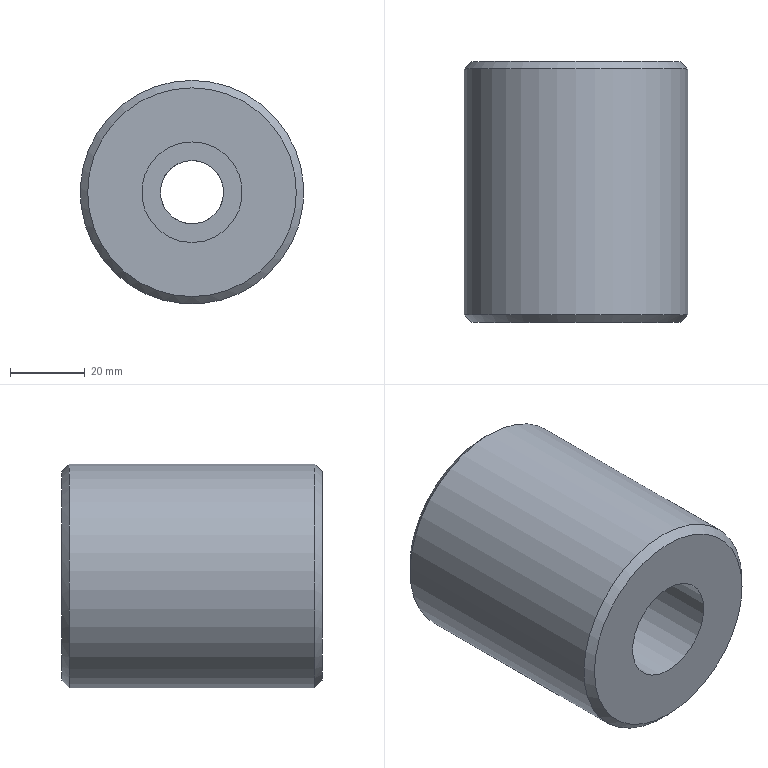Part | STEP file | 车灯-后视镜_id450_x_t | 1 solid | 8 faces | box 60 x 70 x 60 mm | volume 173692 mm3 | plane 3 | cylinder 3 | cone 2 | commonest cylinder face diameters 17 x1 27 x1 60 x1
STEP:
#1=CARTESIAN_POINT('',(165.,-345.,131.5));
#2=VERTEX_POINT('',#1);
#3=CARTESIAN_POINT('',(165.,-345.,159.5));
#4=DIRECTION('',(0.,1.,0.));
#5=DIRECTION('',(0.,0.,-1.));
#6=AXIS2_PLACEMENT_3D('',#3,#4,#5);
#7=CIRCLE('',#6,28.);
#8=EDGE_CURVE('',#2,#2,#7,.T.);
#9=ORIENTED_EDGE('',*,*,#8,.F.);
#10=EDGE_LOOP('',(#9));
#11=FACE_BOUND('',#10,.T.);
#12=CARTESIAN_POINT('',(165.,-345.,146.));
#13=VERTEX_POINT('',#12);
#14=CARTESIAN_POINT('',(165.,-345.,159.5));
#15=DIRECTION('',(0.,1.,0.));
#16=DIRECTION('',(0.,0.,-1.));
#17=AXIS2_PLACEMENT_3D('',#14,#15,#16);
#18=CIRCLE('',#17,13.5);
#19=EDGE_CURVE('',#13,#13,#18,.T.);
#20=ORIENTED_EDGE('',*,*,#19,.T.);
#21=EDGE_LOOP('',(#20));
#22=FACE_BOUND('',#21,.T.);
#23=CARTESIAN_POINT('',(165.,-345.,159.5));
#24=DIRECTION('',(0.,-1.,0.));
#25=DIRECTION('',(0.,0.,-1.));
#26=AXIS2_PLACEMENT_3D('',#23,#24,#25);
#27=PLANE('',#26);
#28=ADVANCED_FACE('',(#11,#22),#27,.T.);
#29=CARTESIAN_POINT('',(165.,-275.,187.5));
#30=VERTEX_POINT('',#29);
#31=CARTESIAN_POINT('',(165.,-275.,159.5));
#32=DIRECTION('',(0.,-1.,0.));
#33=DIRECTION('',(0.,0.,1.));
#34=AXIS2_PLACEMENT_3D('',#31,#32,#33);
#35=CIRCLE('',#34,28.);
#36=EDGE_CURVE('',#30,#30,#35,.T.);
#37=ORIENTED_EDGE('',*,*,#36,.F.);
#38=EDGE_LOOP('',(#37));
#39=FACE_BOUND('',#38,.T.);
#40=CARTESIAN_POINT('',(173.5,-275.,159.5));
#41=VERTEX_POINT('',#40);
#42=CARTESIAN_POINT('',(165.,-275.,159.5));
#43=DIRECTION('',(0.,1.,0.));
#44=DIRECTION('',(1.,0.,0.));
#45=AXIS2_PLACEMENT_3D('',#42,#43,#44);
#46=CIRCLE('',#45,8.5);
#47=EDGE_CURVE('',#41,#41,#46,.T.);
#48=ORIENTED_EDGE('',*,*,#47,.F.);
#49=EDGE_LOOP('',(#48));
#50=FACE_BOUND('',#49,.T.);
#51=CARTESIAN_POINT('',(165.,-275.,159.5));
#52=DIRECTION('',(0.,1.,0.));
#53=DIRECTION('',(0.,0.,1.));
#54=AXIS2_PLACEMENT_3D('',#51,#52,#53);
#55=PLANE('',#54);
#56=ADVANCED_FACE('',(#39,#50),#55,.T.);
#57=CARTESIAN_POINT('',(165.,-277.,189.5));
#58=VERTEX_POINT('',#57);
#59=CARTESIAN_POINT('',(165.,-277.,159.5));
#60=DIRECTION('',(0.,1.,0.));
#61=DIRECTION('',(0.,0.,1.));
#62=AXIS2_PLACEMENT_3D('',#59,#60,#61);
#63=CIRCLE('',#62,30.);
#64=EDGE_CURVE('',#58,#58,#63,.T.);
#65=ORIENTED_EDGE('',*,*,#64,.F.);
#66=EDGE_LOOP('',(#65));
#67=FACE_BOUND('',#66,.T.);
#68=CARTESIAN_POINT('',(165.,-343.,189.5));
#69=VERTEX_POINT('',#68);
#70=CARTESIAN_POINT('',(165.,-343.,159.5));
#71=DIRECTION('',(0.,-1.,0.));
#72=DIRECTION('',(0.,0.,1.));
#73=AXIS2_PLACEMENT_3D('',#70,#71,#72);
#74=CIRCLE('',#73,30.);
#75=EDGE_CURVE('',#69,#69,#74,.T.);
#76=ORIENTED_EDGE('',*,*,#75,.F.);
#77=EDGE_LOOP('',(#76));
#78=FACE_BOUND('',#77,.T.);
#79=CARTESIAN_POINT('',(165.,-275.,159.5));
#80=DIRECTION('',(0.,-1.,0.));
#81=DIRECTION('',(0.,0.,-1.));
#82=AXIS2_PLACEMENT_3D('',#79,#80,#81);
#83=CYLINDRICAL_SURFACE('',#82,30.);
#84=ADVANCED_FACE('',(#67,#78),#83,.T.);
#85=CARTESIAN_POINT('',(165.,-323.,168.));
#86=VERTEX_POINT('',#85);
#87=CARTESIAN_POINT('',(165.,-323.,159.5));
#88=DIRECTION('',(0.,1.,0.));
#89=DIRECTION('',(0.,0.,1.));
#90=AXIS2_PLACEMENT_3D('',#87,#88,#89);
#91=CIRCLE('',#90,8.5);
#92=EDGE_CURVE('',#86,#86,#91,.T.);
#93=ORIENTED_EDGE('',*,*,#92,.F.);
#94=EDGE_LOOP('',(#93));
#95=FACE_BOUND('',#94,.T.);
#96=ORIENTED_EDGE('',*,*,#47,.T.);
#97=EDGE_LOOP('',(#96));
#98=FACE_BOUND('',#97,.T.);
#99=CARTESIAN_POINT('',(165.,-275.,159.5));
#100=DIRECTION('',(0.,-1.,0.));
#101=DIRECTION('',(1.,0.,0.));
#102=AXIS2_PLACEMENT_3D('',#99,#100,#101);
#103=CYLINDRICAL_SURFACE('',#102,8.5);
#104=ADVANCED_FACE('',(#95,#98),#103,.F.);
#105=ORIENTED_EDGE('',*,*,#92,.T.);
#106=EDGE_LOOP('',(#105));
#107=FACE_BOUND('',#106,.T.);
#108=CARTESIAN_POINT('',(165.,-323.,173.));
#109=VERTEX_POINT('',#108);
#110=CARTESIAN_POINT('',(165.,-323.,159.5));
#111=DIRECTION('',(0.,1.,0.));
#112=DIRECTION('',(0.,0.,1.));
#113=AXIS2_PLACEMENT_3D('',#110,#111,#112);
#114=CIRCLE('',#113,13.5);
#115=EDGE_CURVE('',#109,#109,#114,.T.);
#116=ORIENTED_EDGE('',*,*,#115,.F.);
#117=EDGE_LOOP('',(#116));
#118=FACE_BOUND('',#117,.T.);
#119=CARTESIAN_POINT('',(165.,-323.,159.5));
#120=DIRECTION('',(0.,1.,0.));
#121=DIRECTION('',(-1.,0.,0.));
#122=AXIS2_PLACEMENT_3D('',#119,#120,#121);
#123=PLANE('',#122);
#124=ADVANCED_FACE('',(#107,#118),#123,.F.);
#125=ORIENTED_EDGE('',*,*,#19,.F.);
#126=EDGE_LOOP('',(#125));
#127=FACE_BOUND('',#126,.T.);
#128=ORIENTED_EDGE('',*,*,#115,.T.);
#129=EDGE_LOOP('',(#128));
#130=FACE_BOUND('',#129,.T.);
#131=CARTESIAN_POINT('',(165.,-355.,159.5));
#132=DIRECTION('',(0.,1.,0.));
#133=DIRECTION('',(-1.,0.,0.));
#134=AXIS2_PLACEMENT_3D('',#131,#132,#133);
#135=CYLINDRICAL_SURFACE('',#134,13.5);
#136=ADVANCED_FACE('',(#127,#130),#135,.F.);
#137=ORIENTED_EDGE('',*,*,#36,.T.);
#138=EDGE_LOOP('',(#137));
#139=FACE_BOUND('',#138,.T.);
#140=ORIENTED_EDGE('',*,*,#64,.T.);
#141=EDGE_LOOP('',(#140));
#142=FACE_BOUND('',#141,.T.);
#143=CARTESIAN_POINT('',(165.,-277.,159.5));
#144=DIRECTION('',(0.,-1.,0.));
#145=DIRECTION('',(0.,0.,-1.));
#146=AXIS2_PLACEMENT_3D('',#143,#144,#145);
#147=CONICAL_SURFACE('',#146,30.,45.);
#148=ADVANCED_FACE('',(#139,#142),#147,.T.);
#149=ORIENTED_EDGE('',*,*,#8,.T.);
#150=EDGE_LOOP('',(#149));
#151=FACE_BOUND('',#150,.T.);
#152=ORIENTED_EDGE('',*,*,#75,.T.);
#153=EDGE_LOOP('',(#152));
#154=FACE_BOUND('',#153,.T.);
#155=CARTESIAN_POINT('',(165.,-343.,159.5));
#156=DIRECTION('',(0.,1.,0.));
#157=DIRECTION('',(0.,0.,1.));
#158=AXIS2_PLACEMENT_3D('',#155,#156,#157);
#159=CONICAL_SURFACE('',#158,30.,45.);
#160=ADVANCED_FACE('',(#151,#154),#159,.T.);
#161=CLOSED_SHELL('',(#28,#56,#84,#104,#124,#136,#148,#160));
#162=MANIFOLD_SOLID_BREP('',#161);
#163=(LENGTH_UNIT()NAMED_UNIT(*)SI_UNIT(.MILLI.,.METRE.));
#164=UNCERTAINTY_MEASURE_WITH_UNIT(LENGTH_MEASURE(0.00002),#163,'','');
#165=(NAMED_UNIT(*)PLANE_ANGLE_UNIT()SI_UNIT($,.RADIAN.));
#166=PLANE_ANGLE_MEASURE_WITH_UNIT(PLANE_ANGLE_MEASURE(0.01745),#165);
#167=DIMENSIONAL_EXPONENTS(0.,0.,0.,0.,0.,0.,0.);
#168=(CONVERSION_BASED_UNIT('DEGREE',#166)NAMED_UNIT(#167)PLANE_ANGLE_UNIT());
#169=(NAMED_UNIT(*)SI_UNIT($,.STERADIAN.)SOLID_ANGLE_UNIT());
#170=(GEOMETRIC_REPRESENTATION_CONTEXT(3)GLOBAL_UNCERTAINTY_ASSIGNED_CONTEXT((#164))GLOBAL_UNIT_ASSIGNED_CONTEXT((#163,#168,#169))REPRESENTATION_CONTEXT('',''));
#171=ADVANCED_BREP_SHAPE_REPRESENTATION('',(#162),#170);